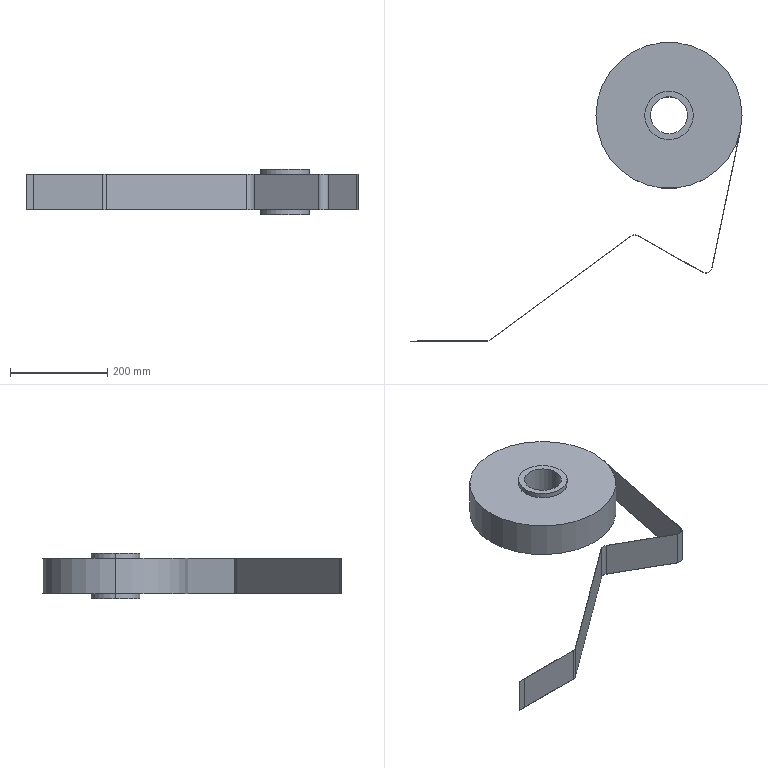Part | STEP file | Transparent bag feed part | 3 solids | 32 faces | box 682 x 614 x 93 mm | volume 4868515 mm3 | plane 18 | cylinder 14 | commonest cylinder face diameters 100 x4 28 x3 27 x2 76 x2 300 x2 29 x1